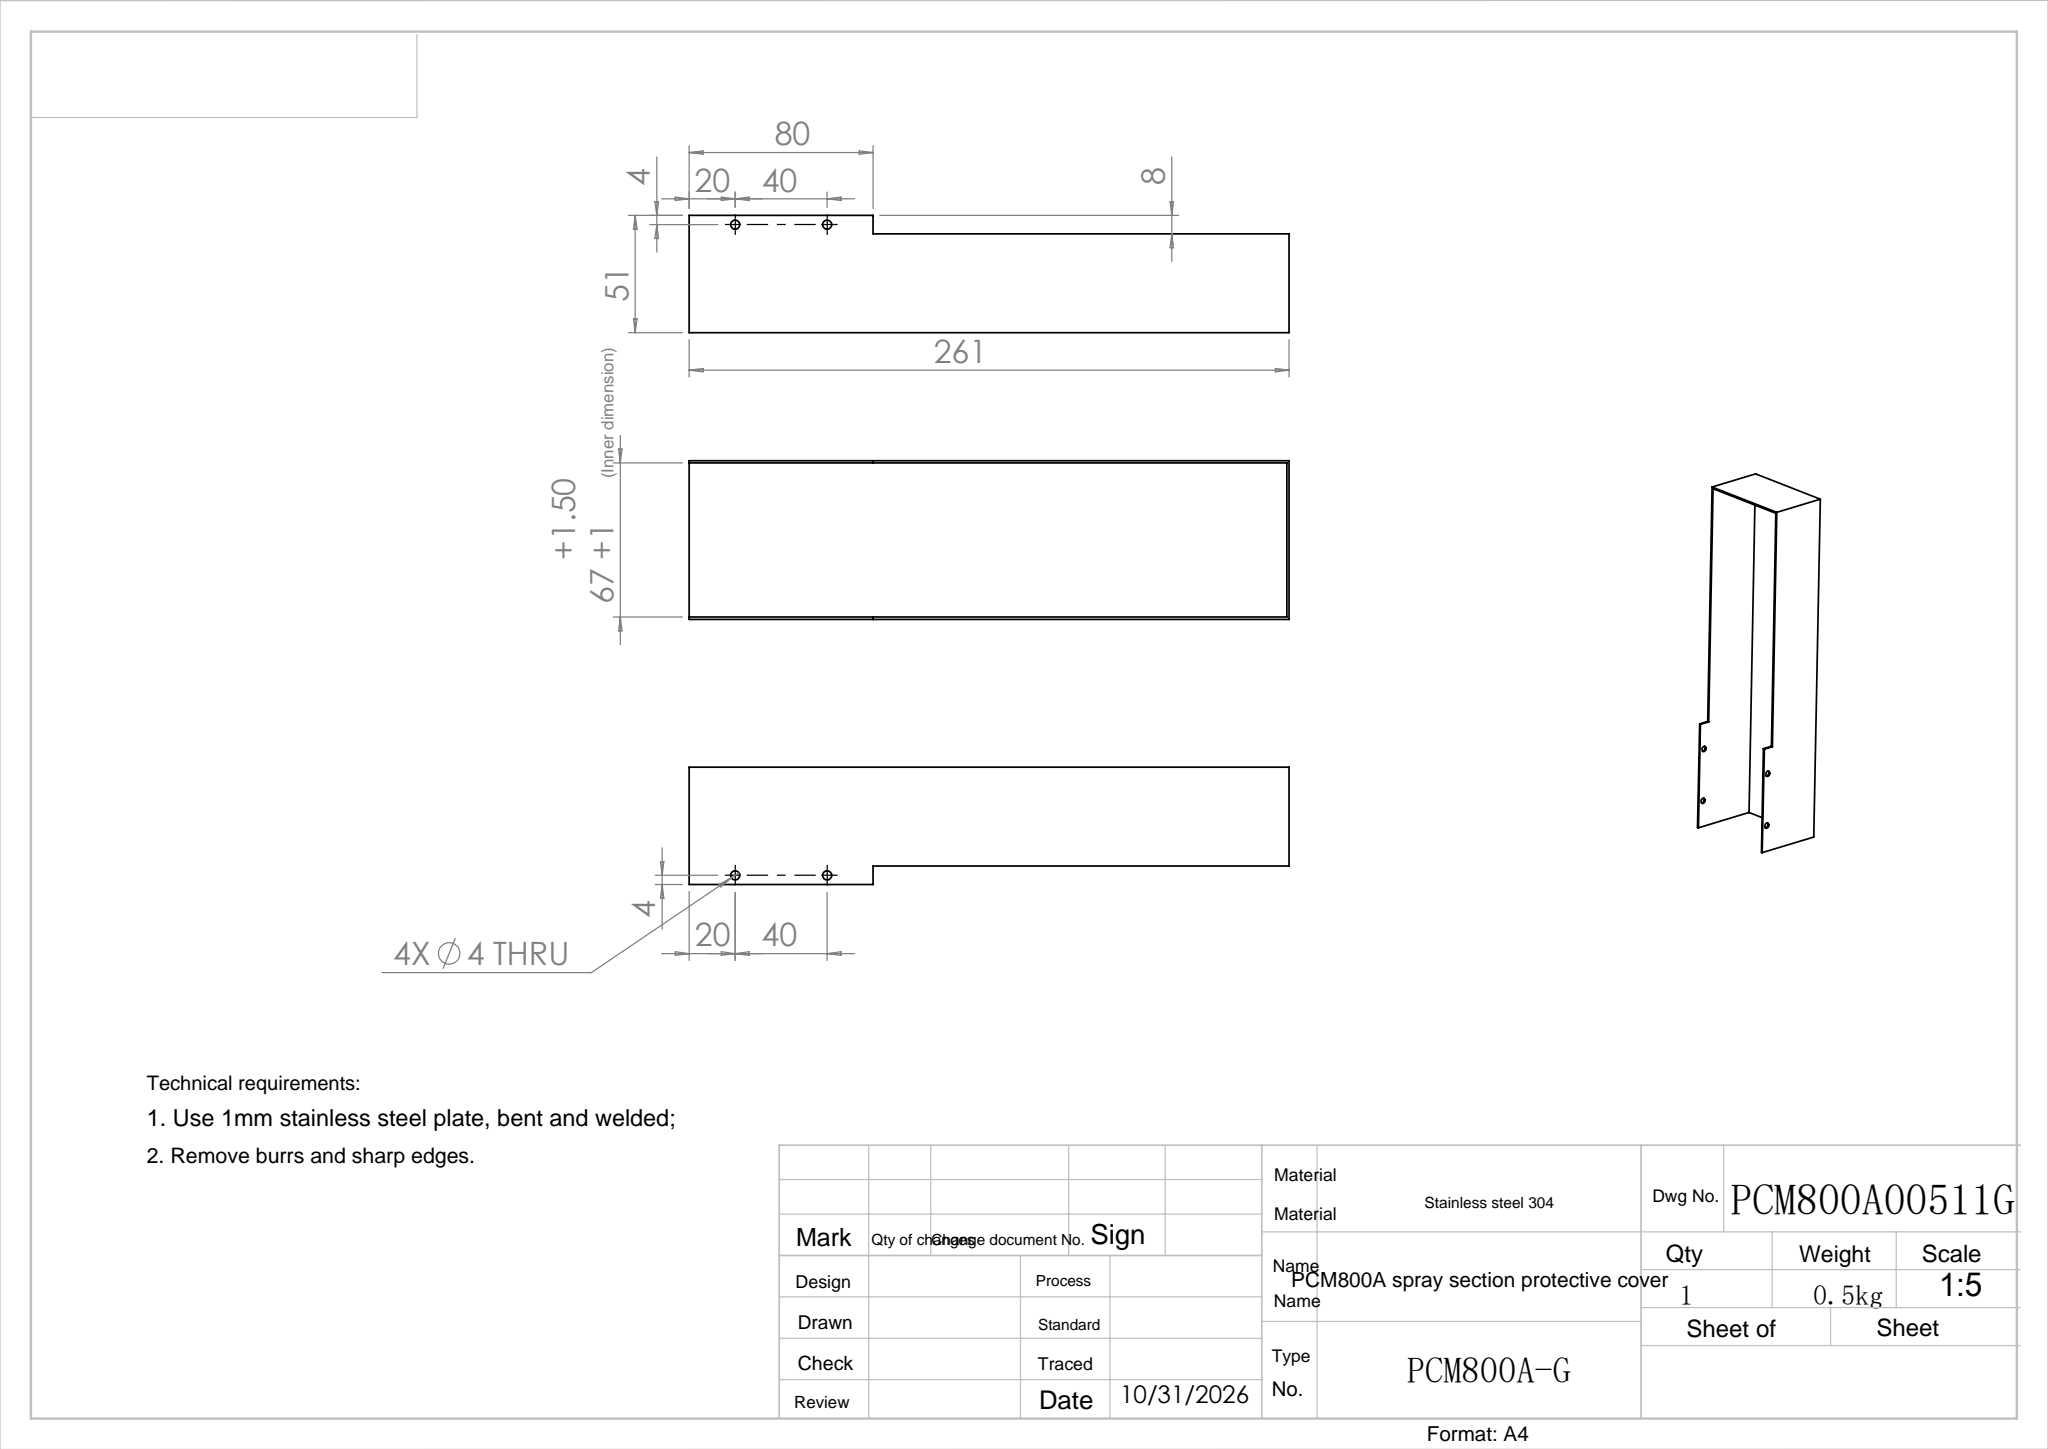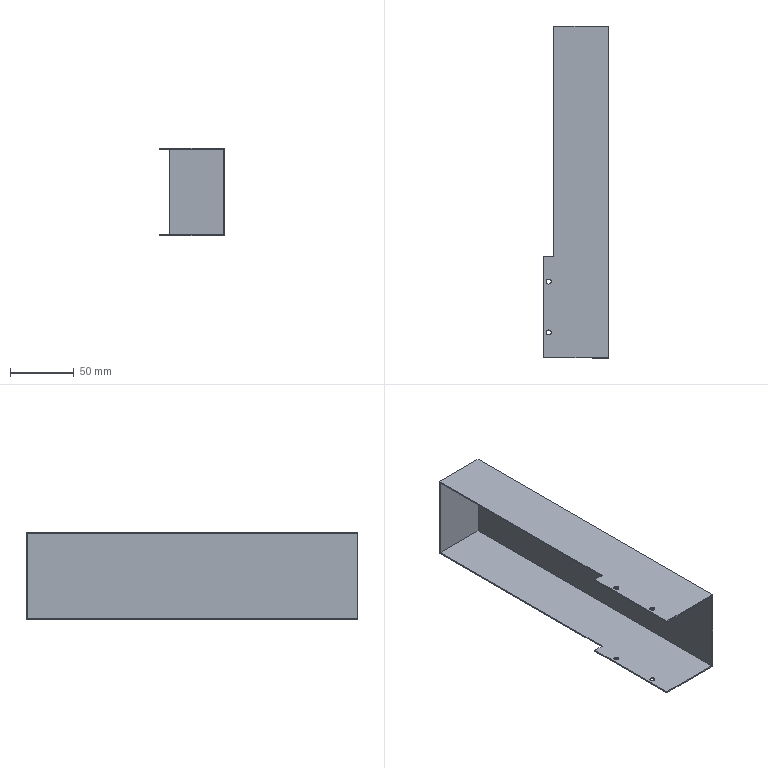Part | SolidWorks | features Extrusion 1, ICE 1, LPattern 1, Shell 1 | 1 solid | 22 faces | box 51 x 261 x 69 mm | volume 43977 mm3 | plane 14 | cylinder 8 | commonest cylinder face diameters 4 x8
STEP:
#1=CARTESIAN_POINT('',(-0.8769,-334.95,67.));
#2=VERTEX_POINT('',#1);
#3=CARTESIAN_POINT('',(3.123,-334.95,67.));
#4=VERTEX_POINT('',#3);
#5=CARTESIAN_POINT('',(1.123,-334.95,67.));
#6=DIRECTION('',(0.,0.,1.));
#7=DIRECTION('',(1.,0.,0.));
#8=AXIS2_PLACEMENT_3D('',#5,#6,#7);
#9=CIRCLE('',#8,2.);
#10=EDGE_CURVE('',#2,#4,#9,.T.);
#11=ORIENTED_EDGE('',*,*,#10,.F.);
#12=CARTESIAN_POINT('',(-0.8769,-334.95,68.));
#13=VERTEX_POINT('',#12);
#14=CARTESIAN_POINT('',(-0.8769,-334.95,-1.));
#15=DIRECTION('',(0.,0.,1.));
#16=VECTOR('',#15,1000.);
#17=LINE('',#14,#16);
#18=EDGE_CURVE('',#2,#13,#17,.T.);
#19=ORIENTED_EDGE('',*,*,#18,.T.);
#20=CARTESIAN_POINT('',(3.123,-334.95,68.));
#21=VERTEX_POINT('',#20);
#22=CARTESIAN_POINT('',(1.123,-334.95,68.));
#23=DIRECTION('',(0.,0.,1.));
#24=DIRECTION('',(1.,0.,0.));
#25=AXIS2_PLACEMENT_3D('',#22,#23,#24);
#26=CIRCLE('',#25,2.);
#27=EDGE_CURVE('',#13,#21,#26,.T.);
#28=ORIENTED_EDGE('',*,*,#27,.T.);
#29=CARTESIAN_POINT('',(3.123,-334.95,-1.));
#30=DIRECTION('',(0.,0.,1.));
#31=VECTOR('',#30,1000.);
#32=LINE('',#29,#31);
#33=EDGE_CURVE('',#4,#21,#32,.T.);
#34=ORIENTED_EDGE('',*,*,#33,.F.);
#35=EDGE_LOOP('',(#11,#19,#28,#34));
#36=FACE_OUTER_BOUND('',#35,.T.);
#37=CARTESIAN_POINT('',(1.123,-334.95,-1.));
#38=DIRECTION('',(0.,0.,1.));
#39=DIRECTION('',(1.,0.,0.));
#40=AXIS2_PLACEMENT_3D('',#37,#38,#39);
#41=CYLINDRICAL_SURFACE('',#40,2.);
#42=ADVANCED_FACE('',(#36),#41,.F.);
#43=CARTESIAN_POINT('',(-0.8769,-334.95,-1.));
#44=VERTEX_POINT('',#43);
#45=CARTESIAN_POINT('',(3.123,-334.95,-1.));
#46=VERTEX_POINT('',#45);
#47=CARTESIAN_POINT('',(1.123,-334.95,-1.));
#48=DIRECTION('',(0.,0.,1.));
#49=DIRECTION('',(1.,0.,0.));
#50=AXIS2_PLACEMENT_3D('',#47,#48,#49);
#51=CIRCLE('',#50,2.);
#52=EDGE_CURVE('',#44,#46,#51,.T.);
#53=ORIENTED_EDGE('',*,*,#52,.F.);
#54=CARTESIAN_POINT('',(-0.8769,-334.95,0.));
#55=VERTEX_POINT('',#54);
#56=CARTESIAN_POINT('',(-0.8769,-334.95,-1.));
#57=DIRECTION('',(0.,0.,1.));
#58=VECTOR('',#57,1000.);
#59=LINE('',#56,#58);
#60=EDGE_CURVE('',#44,#55,#59,.T.);
#61=ORIENTED_EDGE('',*,*,#60,.T.);
#62=CARTESIAN_POINT('',(3.123,-334.95,0.));
#63=VERTEX_POINT('',#62);
#64=CARTESIAN_POINT('',(1.123,-334.95,0.));
#65=DIRECTION('',(0.,0.,1.));
#66=DIRECTION('',(1.,0.,0.));
#67=AXIS2_PLACEMENT_3D('',#64,#65,#66);
#68=CIRCLE('',#67,2.);
#69=EDGE_CURVE('',#55,#63,#68,.T.);
#70=ORIENTED_EDGE('',*,*,#69,.T.);
#71=CARTESIAN_POINT('',(3.123,-334.95,-1.));
#72=DIRECTION('',(0.,0.,1.));
#73=VECTOR('',#72,1000.);
#74=LINE('',#71,#73);
#75=EDGE_CURVE('',#46,#63,#74,.T.);
#76=ORIENTED_EDGE('',*,*,#75,.F.);
#77=EDGE_LOOP('',(#53,#61,#70,#76));
#78=FACE_OUTER_BOUND('',#77,.T.);
#79=CARTESIAN_POINT('',(1.123,-334.95,-1.));
#80=DIRECTION('',(0.,0.,1.));
#81=DIRECTION('',(1.,0.,0.));
#82=AXIS2_PLACEMENT_3D('',#79,#80,#81);
#83=CYLINDRICAL_SURFACE('',#82,2.);
#84=ADVANCED_FACE('',(#78),#83,.F.);
#85=CARTESIAN_POINT('',(-0.8769,-374.95,67.));
#86=VERTEX_POINT('',#85);
#87=CARTESIAN_POINT('',(3.123,-374.95,67.));
#88=VERTEX_POINT('',#87);
#89=CARTESIAN_POINT('',(1.123,-374.95,67.));
#90=DIRECTION('',(0.,0.,1.));
#91=DIRECTION('',(1.,0.,0.));
#92=AXIS2_PLACEMENT_3D('',#89,#90,#91);
#93=CIRCLE('',#92,2.);
#94=EDGE_CURVE('',#86,#88,#93,.T.);
#95=ORIENTED_EDGE('',*,*,#94,.F.);
#96=CARTESIAN_POINT('',(-0.8769,-374.95,68.));
#97=VERTEX_POINT('',#96);
#98=CARTESIAN_POINT('',(-0.8769,-374.95,-1.));
#99=DIRECTION('',(0.,0.,1.));
#100=VECTOR('',#99,1000.);
#101=LINE('',#98,#100);
#102=EDGE_CURVE('',#86,#97,#101,.T.);
#103=ORIENTED_EDGE('',*,*,#102,.T.);
#104=CARTESIAN_POINT('',(3.123,-374.95,68.));
#105=VERTEX_POINT('',#104);
#106=CARTESIAN_POINT('',(1.123,-374.95,68.));
#107=DIRECTION('',(0.,0.,1.));
#108=DIRECTION('',(1.,0.,0.));
#109=AXIS2_PLACEMENT_3D('',#106,#107,#108);
#110=CIRCLE('',#109,2.);
#111=EDGE_CURVE('',#97,#105,#110,.T.);
#112=ORIENTED_EDGE('',*,*,#111,.T.);
#113=CARTESIAN_POINT('',(3.123,-374.95,-1.));
#114=DIRECTION('',(0.,0.,1.));
#115=VECTOR('',#114,1000.);
#116=LINE('',#113,#115);
#117=EDGE_CURVE('',#88,#105,#116,.T.);
#118=ORIENTED_EDGE('',*,*,#117,.F.);
#119=EDGE_LOOP('',(#95,#103,#112,#118));
#120=FACE_OUTER_BOUND('',#119,.T.);
#121=CARTESIAN_POINT('',(1.123,-374.95,-1.));
#122=DIRECTION('',(0.,0.,1.));
#123=DIRECTION('',(1.,0.,0.));
#124=AXIS2_PLACEMENT_3D('',#121,#122,#123);
#125=CYLINDRICAL_SURFACE('',#124,2.);
#126=ADVANCED_FACE('',(#120),#125,.F.);
#127=CARTESIAN_POINT('',(-0.8769,-374.95,-1.));
#128=VERTEX_POINT('',#127);
#129=CARTESIAN_POINT('',(3.123,-374.95,-1.));
#130=VERTEX_POINT('',#129);
#131=CARTESIAN_POINT('',(1.123,-374.95,-1.));
#132=DIRECTION('',(0.,0.,1.));
#133=DIRECTION('',(1.,0.,0.));
#134=AXIS2_PLACEMENT_3D('',#131,#132,#133);
#135=CIRCLE('',#134,2.);
#136=EDGE_CURVE('',#128,#130,#135,.T.);
#137=ORIENTED_EDGE('',*,*,#136,.F.);
#138=CARTESIAN_POINT('',(-0.8769,-374.95,0.));
#139=VERTEX_POINT('',#138);
#140=CARTESIAN_POINT('',(-0.8769,-374.95,-1.));
#141=DIRECTION('',(0.,0.,1.));
#142=VECTOR('',#141,1000.);
#143=LINE('',#140,#142);
#144=EDGE_CURVE('',#128,#139,#143,.T.);
#145=ORIENTED_EDGE('',*,*,#144,.T.);
#146=CARTESIAN_POINT('',(3.123,-374.95,0.));
#147=VERTEX_POINT('',#146);
#148=CARTESIAN_POINT('',(1.123,-374.95,0.));
#149=DIRECTION('',(0.,0.,1.));
#150=DIRECTION('',(1.,0.,0.));
#151=AXIS2_PLACEMENT_3D('',#148,#149,#150);
#152=CIRCLE('',#151,2.);
#153=EDGE_CURVE('',#139,#147,#152,.T.);
#154=ORIENTED_EDGE('',*,*,#153,.T.);
#155=CARTESIAN_POINT('',(3.123,-374.95,-1.));
#156=DIRECTION('',(0.,0.,1.));
#157=VECTOR('',#156,1000.);
#158=LINE('',#155,#157);
#159=EDGE_CURVE('',#130,#147,#158,.T.);
#160=ORIENTED_EDGE('',*,*,#159,.F.);
#161=EDGE_LOOP('',(#137,#145,#154,#160));
#162=FACE_OUTER_BOUND('',#161,.T.);
#163=CARTESIAN_POINT('',(1.123,-374.95,-1.));
#164=DIRECTION('',(0.,0.,1.));
#165=DIRECTION('',(1.,0.,0.));
#166=AXIS2_PLACEMENT_3D('',#163,#164,#165);
#167=CYLINDRICAL_SURFACE('',#166,2.);
#168=ADVANCED_FACE('',(#162),#167,.F.);
#169=CARTESIAN_POINT('',(5.123,-134.95,0.));
#170=VERTEX_POINT('',#169);
#171=CARTESIAN_POINT('',(5.123,-314.95,0.));
#172=VERTEX_POINT('',#171);
#173=CARTESIAN_POINT('',(5.123,-134.95,0.));
#174=DIRECTION('',(0.,-1.,0.));
#175=VECTOR('',#174,1000.);
#176=LINE('',#173,#175);
#177=EDGE_CURVE('',#170,#172,#176,.T.);
#178=ORIENTED_EDGE('',*,*,#177,.F.);
#179=CARTESIAN_POINT('',(5.123,-134.95,67.));
#180=VERTEX_POINT('',#179);
#181=CARTESIAN_POINT('',(5.123,-134.95,67.));
#182=DIRECTION('',(0.,0.,-1.));
#183=VECTOR('',#182,1000.);
#184=LINE('',#181,#183);
#185=EDGE_CURVE('',#180,#170,#184,.T.);
#186=ORIENTED_EDGE('',*,*,#185,.F.);
#187=CARTESIAN_POINT('',(5.123,-314.95,67.));
#188=VERTEX_POINT('',#187);
#189=CARTESIAN_POINT('',(5.123,-134.95,67.));
#190=DIRECTION('',(0.,-1.,0.));
#191=VECTOR('',#190,1000.);
#192=LINE('',#189,#191);
#193=EDGE_CURVE('',#180,#188,#192,.T.);
#194=ORIENTED_EDGE('',*,*,#193,.T.);
#195=CARTESIAN_POINT('',(5.123,-314.95,68.));
#196=VERTEX_POINT('',#195);
#197=CARTESIAN_POINT('',(5.123,-314.95,67.));
#198=DIRECTION('',(0.,0.,-1.));
#199=VECTOR('',#198,1000.);
#200=LINE('',#197,#199);
#201=EDGE_CURVE('',#196,#188,#200,.T.);
#202=ORIENTED_EDGE('',*,*,#201,.F.);
#203=CARTESIAN_POINT('',(5.123,-133.95,68.));
#204=VERTEX_POINT('',#203);
#205=CARTESIAN_POINT('',(5.123,-134.95,68.));
#206=DIRECTION('',(0.,-1.,0.));
#207=VECTOR('',#206,1000.);
#208=LINE('',#205,#207);
#209=EDGE_CURVE('',#204,#196,#208,.T.);
#210=ORIENTED_EDGE('',*,*,#209,.F.);
#211=CARTESIAN_POINT('',(5.123,-133.95,-1.));
#212=VERTEX_POINT('',#211);
#213=CARTESIAN_POINT('',(5.123,-133.95,67.));
#214=DIRECTION('',(0.,0.,-1.));
#215=VECTOR('',#214,1000.);
#216=LINE('',#213,#215);
#217=EDGE_CURVE('',#204,#212,#216,.T.);
#218=ORIENTED_EDGE('',*,*,#217,.T.);
#219=CARTESIAN_POINT('',(5.123,-314.95,-1.));
#220=VERTEX_POINT('',#219);
#221=CARTESIAN_POINT('',(5.123,-134.95,-1.));
#222=DIRECTION('',(0.,-1.,0.));
#223=VECTOR('',#222,1000.);
#224=LINE('',#221,#223);
#225=EDGE_CURVE('',#212,#220,#224,.T.);
#226=ORIENTED_EDGE('',*,*,#225,.T.);
#227=CARTESIAN_POINT('',(5.123,-314.95,67.));
#228=DIRECTION('',(0.,0.,-1.));
#229=VECTOR('',#228,1000.);
#230=LINE('',#227,#229);
#231=EDGE_CURVE('',#172,#220,#230,.T.);
#232=ORIENTED_EDGE('',*,*,#231,.F.);
#233=EDGE_LOOP('',(#178,#186,#194,#202,#210,#218,#226,#232));
#234=FACE_OUTER_BOUND('',#233,.T.);
#235=CARTESIAN_POINT('',(5.123,-134.95,67.));
#236=DIRECTION('',(1.,0.,0.));
#237=DIRECTION('',(0.,1.,0.));
#238=AXIS2_PLACEMENT_3D('',#235,#236,#237);
#239=PLANE('',#238);
#240=ADVANCED_FACE('',(#234),#239,.F.);
#241=CARTESIAN_POINT('',(-2.877,-314.95,0.));
#242=VERTEX_POINT('',#241);
#243=CARTESIAN_POINT('',(5.123,-314.95,0.));
#244=DIRECTION('',(-1.,0.,0.));
#245=VECTOR('',#244,1000.);
#246=LINE('',#243,#245);
#247=EDGE_CURVE('',#172,#242,#246,.T.);
#248=ORIENTED_EDGE('',*,*,#247,.F.);
#249=ORIENTED_EDGE('',*,*,#231,.T.);
#250=CARTESIAN_POINT('',(-2.877,-314.95,-1.));
#251=VERTEX_POINT('',#250);
#252=CARTESIAN_POINT('',(5.123,-314.95,-1.));
#253=DIRECTION('',(-1.,0.,0.));
#254=VECTOR('',#253,1000.);
#255=LINE('',#252,#254);
#256=EDGE_CURVE('',#220,#251,#255,.T.);
#257=ORIENTED_EDGE('',*,*,#256,.T.);
#258=CARTESIAN_POINT('',(-2.877,-314.95,67.));
#259=DIRECTION('',(0.,0.,-1.));
#260=VECTOR('',#259,1000.);
#261=LINE('',#258,#260);
#262=EDGE_CURVE('',#242,#251,#261,.T.);
#263=ORIENTED_EDGE('',*,*,#262,.F.);
#264=EDGE_LOOP('',(#248,#249,#257,#263));
#265=FACE_OUTER_BOUND('',#264,.T.);
#266=CARTESIAN_POINT('',(5.123,-314.95,67.));
#267=DIRECTION('',(0.,-1.,0.));
#268=DIRECTION('',(0.,0.,-1.));
#269=AXIS2_PLACEMENT_3D('',#266,#267,#268);
#270=PLANE('',#269);
#271=ADVANCED_FACE('',(#265),#270,.F.);
#272=CARTESIAN_POINT('',(-2.877,-394.95,0.));
#273=VERTEX_POINT('',#272);
#274=CARTESIAN_POINT('',(-2.877,-314.95,0.));
#275=DIRECTION('',(0.,-1.,0.));
#276=VECTOR('',#275,1000.);
#277=LINE('',#274,#276);
#278=EDGE_CURVE('',#242,#273,#277,.T.);
#279=ORIENTED_EDGE('',*,*,#278,.F.);
#280=ORIENTED_EDGE('',*,*,#262,.T.);
#281=CARTESIAN_POINT('',(-2.877,-394.95,-1.));
#282=VERTEX_POINT('',#281);
#283=CARTESIAN_POINT('',(-2.877,-314.95,-1.));
#284=DIRECTION('',(0.,-1.,0.));
#285=VECTOR('',#284,1000.);
#286=LINE('',#283,#285);
#287=EDGE_CURVE('',#251,#282,#286,.T.);
#288=ORIENTED_EDGE('',*,*,#287,.T.);
#289=CARTESIAN_POINT('',(-2.877,-394.95,67.));
#290=DIRECTION('',(0.,0.,-1.));
#291=VECTOR('',#290,1000.);
#292=LINE('',#289,#291);
#293=EDGE_CURVE('',#273,#282,#292,.T.);
#294=ORIENTED_EDGE('',*,*,#293,.F.);
#295=EDGE_LOOP('',(#279,#280,#288,#294));
#296=FACE_OUTER_BOUND('',#295,.T.);
#297=CARTESIAN_POINT('',(-2.877,-314.95,67.));
#298=DIRECTION('',(1.,0.,0.));
#299=DIRECTION('',(0.,1.,0.));
#300=AXIS2_PLACEMENT_3D('',#297,#298,#299);
#301=PLANE('',#300);
#302=ADVANCED_FACE('',(#296),#301,.F.);
#303=CARTESIAN_POINT('',(47.123,-394.95,0.));
#304=VERTEX_POINT('',#303);
#305=CARTESIAN_POINT('',(-2.877,-394.95,0.));
#306=DIRECTION('',(1.,0.,0.));
#307=VECTOR('',#306,1000.);
#308=LINE('',#305,#307);
#309=EDGE_CURVE('',#273,#304,#308,.T.);
#310=ORIENTED_EDGE('',*,*,#309,.F.);
#311=ORIENTED_EDGE('',*,*,#293,.T.);
#312=CARTESIAN_POINT('',(48.123,-394.95,-1.));
#313=VERTEX_POINT('',#312);
#314=CARTESIAN_POINT('',(-2.877,-394.95,-1.));
#315=DIRECTION('',(1.,0.,0.));
#316=VECTOR('',#315,1000.);
#317=LINE('',#314,#316);
#318=EDGE_CURVE('',#282,#313,#317,.T.);
#319=ORIENTED_EDGE('',*,*,#318,.T.);
#320=CARTESIAN_POINT('',(48.123,-394.95,68.));
#321=VERTEX_POINT('',#320);
#322=CARTESIAN_POINT('',(48.123,-394.95,67.));
#323=DIRECTION('',(0.,0.,-1.));
#324=VECTOR('',#323,1000.);
#325=LINE('',#322,#324);
#326=EDGE_CURVE('',#321,#313,#325,.T.);
#327=ORIENTED_EDGE('',*,*,#326,.F.);
#328=CARTESIAN_POINT('',(-2.877,-394.95,68.));
#329=VERTEX_POINT('',#328);
#330=CARTESIAN_POINT('',(-2.877,-394.95,68.));
#331=DIRECTION('',(1.,0.,0.));
#332=VECTOR('',#331,1000.);
#333=LINE('',#330,#332);
#334=EDGE_CURVE('',#329,#321,#333,.T.);
#335=ORIENTED_EDGE('',*,*,#334,.F.);
#336=CARTESIAN_POINT('',(-2.877,-394.95,67.));
#337=VERTEX_POINT('',#336);
#338=CARTESIAN_POINT('',(-2.877,-394.95,67.));
#339=DIRECTION('',(0.,0.,-1.));
#340=VECTOR('',#339,1000.);
#341=LINE('',#338,#340);
#342=EDGE_CURVE('',#329,#337,#341,.T.);
#343=ORIENTED_EDGE('',*,*,#342,.T.);
#344=CARTESIAN_POINT('',(47.123,-394.95,67.));
#345=VERTEX_POINT('',#344);
#346=CARTESIAN_POINT('',(-2.877,-394.95,67.));
#347=DIRECTION('',(1.,0.,0.));
#348=VECTOR('',#347,1000.);
#349=LINE('',#346,#348);
#350=EDGE_CURVE('',#337,#345,#349,.T.);
#351=ORIENTED_EDGE('',*,*,#350,.T.);
#352=CARTESIAN_POINT('',(47.123,-394.95,67.));
#353=DIRECTION('',(0.,0.,-1.));
#354=VECTOR('',#353,1000.);
#355=LINE('',#352,#354);
#356=EDGE_CURVE('',#345,#304,#355,.T.);
#357=ORIENTED_EDGE('',*,*,#356,.T.);
#358=EDGE_LOOP('',(#310,#311,#319,#327,#335,#343,#351,#357));
#359=FACE_OUTER_BOUND('',#358,.T.);
#360=CARTESIAN_POINT('',(-2.877,-394.95,67.));
#361=DIRECTION('',(0.,1.,0.));
#362=DIRECTION('',(-1.,0.,0.));
#363=AXIS2_PLACEMENT_3D('',#360,#361,#362);
#364=PLANE('',#363);
#365=ADVANCED_FACE('',(#359),#364,.F.);
#366=CARTESIAN_POINT('',(48.123,-133.95,-1.));
#367=VERTEX_POINT('',#366);
#368=CARTESIAN_POINT('',(48.123,-134.95,-1.));
#369=DIRECTION('',(0.,1.,0.));
#370=VECTOR('',#369,1000.);
#371=LINE('',#368,#370);
#372=EDGE_CURVE('',#313,#367,#371,.T.);
#373=ORIENTED_EDGE('',*,*,#372,.T.);
#374=CARTESIAN_POINT('',(48.123,-133.95,68.));
#375=VERTEX_POINT('',#374);
#376=CARTESIAN_POINT('',(48.123,-133.95,67.));
#377=DIRECTION('',(0.,0.,-1.));
#378=VECTOR('',#377,1000.);
#379=LINE('',#376,#378);
#380=EDGE_CURVE('',#375,#367,#379,.T.);
#381=ORIENTED_EDGE('',*,*,#380,.F.);
#382=CARTESIAN_POINT('',(48.123,-134.95,68.));
#383=DIRECTION('',(0.,1.,0.));
#384=VECTOR('',#383,1000.);
#385=LINE('',#382,#384);
#386=EDGE_CURVE('',#321,#375,#385,.T.);
#387=ORIENTED_EDGE('',*,*,#386,.F.);
#388=ORIENTED_EDGE('',*,*,#326,.T.);
#389=EDGE_LOOP('',(#373,#381,#387,#388));
#390=FACE_OUTER_BOUND('',#389,.T.);
#391=CARTESIAN_POINT('',(48.123,-134.95,67.));
#392=DIRECTION('',(-1.,0.,0.));
#393=DIRECTION('',(0.,-1.,0.));
#394=AXIS2_PLACEMENT_3D('',#391,#392,#393);
#395=PLANE('',#394);
#396=ADVANCED_FACE('',(#390),#395,.F.);
#397=CARTESIAN_POINT('',(5.123,-133.95,-1.));
#398=DIRECTION('',(-1.,0.,0.));
#399=VECTOR('',#398,1000.);
#400=LINE('',#397,#399);
#401=EDGE_CURVE('',#367,#212,#400,.T.);
#402=ORIENTED_EDGE('',*,*,#401,.T.);
#403=ORIENTED_EDGE('',*,*,#217,.F.);
#404=CARTESIAN_POINT('',(5.123,-133.95,68.));
#405=DIRECTION('',(-1.,0.,0.));
#406=VECTOR('',#405,1000.);
#407=LINE('',#404,#406);
#408=EDGE_CURVE('',#375,#204,#407,.T.);
#409=ORIENTED_EDGE('',*,*,#408,.F.);
#410=ORIENTED_EDGE('',*,*,#380,.T.);
#411=EDGE_LOOP('',(#402,#403,#409,#410));
#412=FACE_OUTER_BOUND('',#411,.T.);
#413=CARTESIAN_POINT('',(5.123,-133.95,67.));
#414=DIRECTION('',(0.,-1.,0.));
#415=DIRECTION('',(0.,0.,-1.));
#416=AXIS2_PLACEMENT_3D('',#413,#414,#415);
#417=PLANE('',#416);
#418=ADVANCED_FACE('',(#412),#417,.F.);
#419=ORIENTED_EDGE('',*,*,#201,.T.);
#420=CARTESIAN_POINT('',(-2.877,-314.95,67.));
#421=VERTEX_POINT('',#420);
#422=CARTESIAN_POINT('',(5.123,-314.95,67.));
#423=DIRECTION('',(-1.,0.,0.));
#424=VECTOR('',#423,1000.);
#425=LINE('',#422,#424);
#426=EDGE_CURVE('',#188,#421,#425,.T.);
#427=ORIENTED_EDGE('',*,*,#426,.T.);
#428=CARTESIAN_POINT('',(-2.877,-314.95,68.));
#429=VERTEX_POINT('',#428);
#430=CARTESIAN_POINT('',(-2.877,-314.95,67.));
#431=DIRECTION('',(0.,0.,-1.));
#432=VECTOR('',#431,1000.);
#433=LINE('',#430,#432);
#434=EDGE_CURVE('',#429,#421,#433,.T.);
#435=ORIENTED_EDGE('',*,*,#434,.F.);
#436=CARTESIAN_POINT('',(5.123,-314.95,68.));
#437=DIRECTION('',(-1.,0.,0.));
#438=VECTOR('',#437,1000.);
#439=LINE('',#436,#438);
#440=EDGE_CURVE('',#196,#429,#439,.T.);
#441=ORIENTED_EDGE('',*,*,#440,.F.);
#442=EDGE_LOOP('',(#419,#427,#435,#441));
#443=FACE_OUTER_BOUND('',#442,.T.);
#444=CARTESIAN_POINT('',(5.123,-314.95,67.));
#445=DIRECTION('',(0.,-1.,0.));
#446=DIRECTION('',(0.,0.,-1.));
#447=AXIS2_PLACEMENT_3D('',#444,#445,#446);
#448=PLANE('',#447);
#449=ADVANCED_FACE('',(#443),#448,.F.);
#450=ORIENTED_EDGE('',*,*,#434,.T.);
#451=CARTESIAN_POINT('',(-2.877,-314.95,67.));
#452=DIRECTION('',(0.,-1.,0.));
#453=VECTOR('',#452,1000.);
#454=LINE('',#451,#453);
#455=EDGE_CURVE('',#421,#337,#454,.T.);
#456=ORIENTED_EDGE('',*,*,#455,.T.);
#457=ORIENTED_EDGE('',*,*,#342,.F.);
#458=CARTESIAN_POINT('',(-2.877,-314.95,68.));
#459=DIRECTION('',(0.,-1.,0.));
#460=VECTOR('',#459,1000.);
#461=LINE('',#458,#460);
#462=EDGE_CURVE('',#429,#329,#461,.T.);
#463=ORIENTED_EDGE('',*,*,#462,.F.);
#464=EDGE_LOOP('',(#450,#456,#457,#463));
#465=FACE_OUTER_BOUND('',#464,.T.);
#466=CARTESIAN_POINT('',(-2.877,-314.95,67.));
#467=DIRECTION('',(1.,0.,0.));
#468=DIRECTION('',(0.,1.,0.));
#469=AXIS2_PLACEMENT_3D('',#466,#467,#468);
#470=PLANE('',#469);
#471=ADVANCED_FACE('',(#465),#470,.F.);
#472=CARTESIAN_POINT('',(1.123,-334.95,68.));
#473=DIRECTION('',(0.,0.,1.));
#474=DIRECTION('',(1.,0.,0.));
#475=AXIS2_PLACEMENT_3D('',#472,#473,#474);
#476=CIRCLE('',#475,2.);
#477=EDGE_CURVE('',#21,#13,#476,.T.);
#478=ORIENTED_EDGE('',*,*,#477,.F.);
#479=ORIENTED_EDGE('',*,*,#27,.F.);
#480=EDGE_LOOP('',(#478,#479));
#481=FACE_BOUND('',#480,.T.);
#482=CARTESIAN_POINT('',(1.123,-374.95,68.));
#483=DIRECTION('',(0.,0.,1.));
#484=DIRECTION('',(1.,0.,0.));
#485=AXIS2_PLACEMENT_3D('',#482,#483,#484);
#486=CIRCLE('',#485,2.);
#487=EDGE_CURVE('',#105,#97,#486,.T.);
#488=ORIENTED_EDGE('',*,*,#487,.F.);
#489=ORIENTED_EDGE('',*,*,#111,.F.);
#490=EDGE_LOOP('',(#488,#489));
#491=FACE_BOUND('',#490,.T.);
#492=ORIENTED_EDGE('',*,*,#386,.T.);
#493=ORIENTED_EDGE('',*,*,#408,.T.);
#494=ORIENTED_EDGE('',*,*,#209,.T.);
#495=ORIENTED_EDGE('',*,*,#440,.T.);
#496=ORIENTED_EDGE('',*,*,#462,.T.);
#497=ORIENTED_EDGE('',*,*,#334,.T.);
#498=EDGE_LOOP('',(#492,#493,#494,#495,#496,#497));
#499=FACE_OUTER_BOUND('',#498,.T.);
#500=CARTESIAN_POINT('',(47.123,-394.95,68.));
#501=DIRECTION('',(0.,0.,1.));
#502=DIRECTION('',(1.,0.,0.));
#503=AXIS2_PLACEMENT_3D('',#500,#501,#502);
#504=PLANE('',#503);
#505=ADVANCED_FACE('',(#481,#491,#499),#504,.T.);
#506=CARTESIAN_POINT('',(1.123,-334.95,-1.));
#507=DIRECTION('',(0.,0.,1.));
#508=DIRECTION('',(1.,0.,0.));
#509=AXIS2_PLACEMENT_3D('',#506,#507,#508);
#510=CIRCLE('',#509,2.);
#511=EDGE_CURVE('',#46,#44,#510,.T.);
#512=ORIENTED_EDGE('',*,*,#511,.T.);
#513=ORIENTED_EDGE('',*,*,#52,.T.);
#514=EDGE_LOOP('',(#512,#513));
#515=FACE_BOUND('',#514,.T.);
#516=CARTESIAN_POINT('',(1.123,-374.95,-1.));
#517=DIRECTION('',(0.,0.,1.));
#518=DIRECTION('',(1.,0.,0.));
#519=AXIS2_PLACEMENT_3D('',#516,#517,#518);
#520=CIRCLE('',#519,2.);
#521=EDGE_CURVE('',#130,#128,#520,.T.);
#522=ORIENTED_EDGE('',*,*,#521,.T.);
#523=ORIENTED_EDGE('',*,*,#136,.T.);
#524=EDGE_LOOP('',(#522,#523));
#525=FACE_BOUND('',#524,.T.);
#526=ORIENTED_EDGE('',*,*,#372,.F.);
#527=ORIENTED_EDGE('',*,*,#318,.F.);
#528=ORIENTED_EDGE('',*,*,#287,.F.);
#529=ORIENTED_EDGE('',*,*,#256,.F.);
#530=ORIENTED_EDGE('',*,*,#225,.F.);
#531=ORIENTED_EDGE('',*,*,#401,.F.);
#532=EDGE_LOOP('',(#526,#527,#528,#529,#530,#531));
#533=FACE_OUTER_BOUND('',#532,.T.);
#534=CARTESIAN_POINT('',(47.123,-394.95,-1.));
#535=DIRECTION('',(0.,0.,1.));
#536=DIRECTION('',(1.,0.,0.));
#537=AXIS2_PLACEMENT_3D('',#534,#535,#536);
#538=PLANE('',#537);
#539=ADVANCED_FACE('',(#515,#525,#533),#538,.F.);
#540=CARTESIAN_POINT('',(47.123,-134.95,0.));
#541=VERTEX_POINT('',#540);
#542=CARTESIAN_POINT('',(47.123,-134.95,0.));
#543=DIRECTION('',(0.,1.,0.));
#544=VECTOR('',#543,1000.);
#545=LINE('',#542,#544);
#546=EDGE_CURVE('',#304,#541,#545,.T.);
#547=ORIENTED_EDGE('',*,*,#546,.F.);
#548=ORIENTED_EDGE('',*,*,#356,.F.);
#549=CARTESIAN_POINT('',(47.123,-134.95,67.));
#550=VERTEX_POINT('',#549);
#551=CARTESIAN_POINT('',(47.123,-134.95,67.));
#552=DIRECTION('',(0.,1.,0.));
#553=VECTOR('',#552,1000.);
#554=LINE('',#551,#553);
#555=EDGE_CURVE('',#345,#550,#554,.T.);
#556=ORIENTED_EDGE('',*,*,#555,.T.);
#557=CARTESIAN_POINT('',(47.123,-134.95,67.));
#558=DIRECTION('',(0.,0.,-1.));
#559=VECTOR('',#558,1000.);
#560=LINE('',#557,#559);
#561=EDGE_CURVE('',#550,#541,#560,.T.);
#562=ORIENTED_EDGE('',*,*,#561,.T.);
#563=EDGE_LOOP('',(#547,#548,#556,#562));
#564=FACE_OUTER_BOUND('',#563,.T.);
#565=CARTESIAN_POINT('',(47.123,-134.95,67.));
#566=DIRECTION('',(-1.,0.,0.));
#567=DIRECTION('',(0.,-1.,0.));
#568=AXIS2_PLACEMENT_3D('',#565,#566,#567);
#569=PLANE('',#568);
#570=ADVANCED_FACE('',(#564),#569,.T.);
#571=CARTESIAN_POINT('',(5.123,-134.95,0.));
#572=DIRECTION('',(-1.,0.,0.));
#573=VECTOR('',#572,1000.);
#574=LINE('',#571,#573);
#575=EDGE_CURVE('',#541,#170,#574,.T.);
#576=ORIENTED_EDGE('',*,*,#575,.F.);
#577=ORIENTED_EDGE('',*,*,#561,.F.);
#578=CARTESIAN_POINT('',(5.123,-134.95,67.));
#579=DIRECTION('',(-1.,0.,0.));
#580=VECTOR('',#579,1000.);
#581=LINE('',#578,#580);
#582=EDGE_CURVE('',#550,#180,#581,.T.);
#583=ORIENTED_EDGE('',*,*,#582,.T.);
#584=ORIENTED_EDGE('',*,*,#185,.T.);
#585=EDGE_LOOP('',(#576,#577,#583,#584));
#586=FACE_OUTER_BOUND('',#585,.T.);
#587=CARTESIAN_POINT('',(5.123,-134.95,67.));
#588=DIRECTION('',(0.,-1.,0.));
#589=DIRECTION('',(0.,0.,-1.));
#590=AXIS2_PLACEMENT_3D('',#587,#588,#589);
#591=PLANE('',#590);
#592=ADVANCED_FACE('',(#586),#591,.T.);
#593=CARTESIAN_POINT('',(1.123,-334.95,67.));
#594=DIRECTION('',(0.,0.,1.));
#595=DIRECTION('',(1.,0.,0.));
#596=AXIS2_PLACEMENT_3D('',#593,#594,#595);
#597=CIRCLE('',#596,2.);
#598=EDGE_CURVE('',#4,#2,#597,.T.);
#599=ORIENTED_EDGE('',*,*,#598,.T.);
#600=ORIENTED_EDGE('',*,*,#10,.T.);
#601=EDGE_LOOP('',(#599,#600));
#602=FACE_BOUND('',#601,.T.);
#603=CARTESIAN_POINT('',(1.123,-374.95,67.));
#604=DIRECTION('',(0.,0.,1.));
#605=DIRECTION('',(1.,0.,0.));
#606=AXIS2_PLACEMENT_3D('',#603,#604,#605);
#607=CIRCLE('',#606,2.);
#608=EDGE_CURVE('',#88,#86,#607,.T.);
#609=ORIENTED_EDGE('',*,*,#608,.T.);
#610=ORIENTED_EDGE('',*,*,#94,.T.);
#611=EDGE_LOOP('',(#609,#610));
#612=FACE_BOUND('',#611,.T.);
#613=ORIENTED_EDGE('',*,*,#555,.F.);
#614=ORIENTED_EDGE('',*,*,#350,.F.);
#615=ORIENTED_EDGE('',*,*,#455,.F.);
#616=ORIENTED_EDGE('',*,*,#426,.F.);
#617=ORIENTED_EDGE('',*,*,#193,.F.);
#618=ORIENTED_EDGE('',*,*,#582,.F.);
#619=EDGE_LOOP('',(#613,#614,#615,#616,#617,#618));
#620=FACE_OUTER_BOUND('',#619,.T.);
#621=CARTESIAN_POINT('',(47.123,-394.95,67.));
#622=DIRECTION('',(0.,0.,1.));
#623=DIRECTION('',(1.,0.,0.));
#624=AXIS2_PLACEMENT_3D('',#621,#622,#623);
#625=PLANE('',#624);
#626=ADVANCED_FACE('',(#602,#612,#620),#625,.F.);
#627=CARTESIAN_POINT('',(1.123,-334.95,0.));
#628=DIRECTION('',(0.,0.,1.));
#629=DIRECTION('',(1.,0.,0.));
#630=AXIS2_PLACEMENT_3D('',#627,#628,#629);
#631=CIRCLE('',#630,2.);
#632=EDGE_CURVE('',#63,#55,#631,.T.);
#633=ORIENTED_EDGE('',*,*,#632,.F.);
#634=ORIENTED_EDGE('',*,*,#69,.F.);
#635=EDGE_LOOP('',(#633,#634));
#636=FACE_BOUND('',#635,.T.);
#637=CARTESIAN_POINT('',(1.123,-374.95,0.));
#638=DIRECTION('',(0.,0.,1.));
#639=DIRECTION('',(1.,0.,0.));
#640=AXIS2_PLACEMENT_3D('',#637,#638,#639);
#641=CIRCLE('',#640,2.);
#642=EDGE_CURVE('',#147,#139,#641,.T.);
#643=ORIENTED_EDGE('',*,*,#642,.F.);
#644=ORIENTED_EDGE('',*,*,#153,.F.);
#645=EDGE_LOOP('',(#643,#644));
#646=FACE_BOUND('',#645,.T.);
#647=ORIENTED_EDGE('',*,*,#546,.T.);
#648=ORIENTED_EDGE('',*,*,#575,.T.);
#649=ORIENTED_EDGE('',*,*,#177,.T.);
#650=ORIENTED_EDGE('',*,*,#247,.T.);
#651=ORIENTED_EDGE('',*,*,#278,.T.);
#652=ORIENTED_EDGE('',*,*,#309,.T.);
#653=EDGE_LOOP('',(#647,#648,#649,#650,#651,#652));
#654=FACE_OUTER_BOUND('',#653,.T.);
#655=CARTESIAN_POINT('',(47.123,-394.95,0.));
#656=DIRECTION('',(0.,0.,1.));
#657=DIRECTION('',(1.,0.,0.));
#658=AXIS2_PLACEMENT_3D('',#655,#656,#657);
#659=PLANE('',#658);
#660=ADVANCED_FACE('',(#636,#646,#654),#659,.T.);
#661=ORIENTED_EDGE('',*,*,#144,.F.);
#662=ORIENTED_EDGE('',*,*,#521,.F.);
#663=ORIENTED_EDGE('',*,*,#159,.T.);
#664=ORIENTED_EDGE('',*,*,#642,.T.);
#665=EDGE_LOOP('',(#661,#662,#663,#664));
#666=FACE_OUTER_BOUND('',#665,.T.);
#667=CARTESIAN_POINT('',(1.123,-374.95,-1.));
#668=DIRECTION('',(0.,0.,1.));
#669=DIRECTION('',(1.,0.,0.));
#670=AXIS2_PLACEMENT_3D('',#667,#668,#669);
#671=CYLINDRICAL_SURFACE('',#670,2.);
#672=ADVANCED_FACE('',(#666),#671,.F.);
#673=ORIENTED_EDGE('',*,*,#102,.F.);
#674=ORIENTED_EDGE('',*,*,#608,.F.);
#675=ORIENTED_EDGE('',*,*,#117,.T.);
#676=ORIENTED_EDGE('',*,*,#487,.T.);
#677=EDGE_LOOP('',(#673,#674,#675,#676));
#678=FACE_OUTER_BOUND('',#677,.T.);
#679=CARTESIAN_POINT('',(1.123,-374.95,-1.));
#680=DIRECTION('',(0.,0.,1.));
#681=DIRECTION('',(1.,0.,0.));
#682=AXIS2_PLACEMENT_3D('',#679,#680,#681);
#683=CYLINDRICAL_SURFACE('',#682,2.);
#684=ADVANCED_FACE('',(#678),#683,.F.);
#685=ORIENTED_EDGE('',*,*,#60,.F.);
#686=ORIENTED_EDGE('',*,*,#511,.F.);
#687=ORIENTED_EDGE('',*,*,#75,.T.);
#688=ORIENTED_EDGE('',*,*,#632,.T.);
#689=EDGE_LOOP('',(#685,#686,#687,#688));
#690=FACE_OUTER_BOUND('',#689,.T.);
#691=CARTESIAN_POINT('',(1.123,-334.95,-1.));
#692=DIRECTION('',(0.,0.,1.));
#693=DIRECTION('',(1.,0.,0.));
#694=AXIS2_PLACEMENT_3D('',#691,#692,#693);
#695=CYLINDRICAL_SURFACE('',#694,2.);
#696=ADVANCED_FACE('',(#690),#695,.F.);
#697=ORIENTED_EDGE('',*,*,#18,.F.);
#698=ORIENTED_EDGE('',*,*,#598,.F.);
#699=ORIENTED_EDGE('',*,*,#33,.T.);
#700=ORIENTED_EDGE('',*,*,#477,.T.);
#701=EDGE_LOOP('',(#697,#698,#699,#700));
#702=FACE_OUTER_BOUND('',#701,.T.);
#703=CARTESIAN_POINT('',(1.123,-334.95,-1.));
#704=DIRECTION('',(0.,0.,1.));
#705=DIRECTION('',(1.,0.,0.));
#706=AXIS2_PLACEMENT_3D('',#703,#704,#705);
#707=CYLINDRICAL_SURFACE('',#706,2.);
#708=ADVANCED_FACE('',(#702),#707,.F.);
#709=CLOSED_SHELL('',(#42,#84,#126,#168,#240,#271,#302,#365,#396,#418,#449,#471,#505,#539,#570,#592,#626,#660,#672,#684,#696,#708));
#710=MANIFOLD_SOLID_BREP('',#709);
#711=CARTESIAN_POINT('',(0.,0.,0.));
#712=DIRECTION('',(0.,0.,1.));
#713=DIRECTION('',(1.,0.,0.));
#714=AXIS2_PLACEMENT_3D('',#711,#712,#713);
#715=(LENGTH_UNIT()NAMED_UNIT(*)SI_UNIT(.MILLI.,.METRE.));
#716=UNCERTAINTY_MEASURE_WITH_UNIT(LENGTH_MEASURE(0.00001),#715,'','');
#717=(NAMED_UNIT(*)PLANE_ANGLE_UNIT()SI_UNIT($,.RADIAN.));
#718=(NAMED_UNIT(*)SI_UNIT($,.STERADIAN.)SOLID_ANGLE_UNIT());
#719=(GEOMETRIC_REPRESENTATION_CONTEXT(3)GLOBAL_UNCERTAINTY_ASSIGNED_CONTEXT((#716))GLOBAL_UNIT_ASSIGNED_CONTEXT((#715,#717,#718))REPRESENTATION_CONTEXT('',''));
#720=ADVANCED_BREP_SHAPE_REPRESENTATION('',(#710,#714),#719);